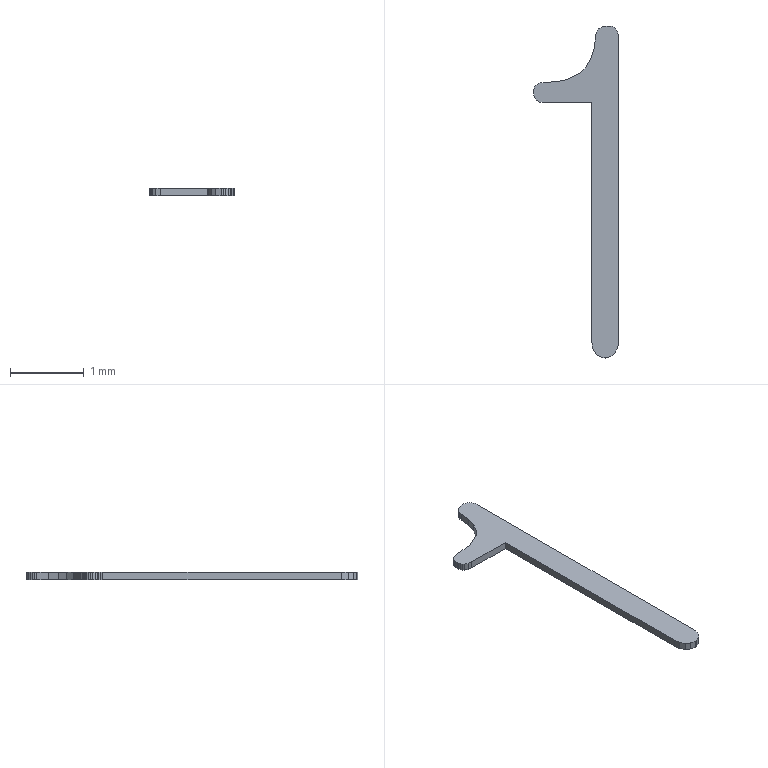Part | STEP file | PART245.stp | 1 solid | 51 faces | box 1.148 x 4.493 x 0.1 mm | volume 0.1844 mm3 | plane 51